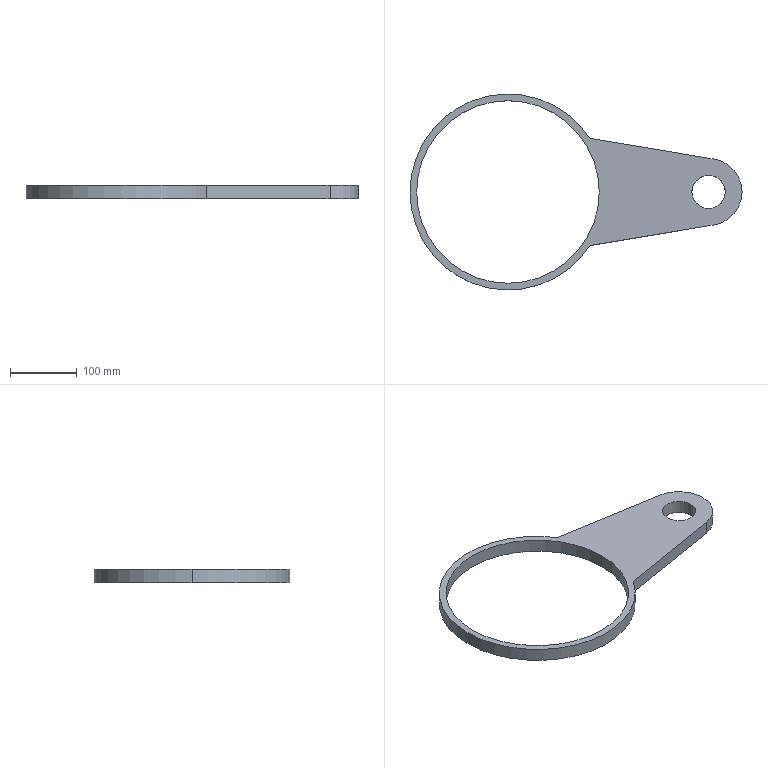Part | SolidWorks | features Extrusion 1 | 1 solid | 11 faces | box 496.5 x 293 x 20 mm | volume 628876 mm3 | cylinder 7 | plane 4 | commonest cylinder face diameters 50 x2 273 x2 293 x2 100 x1
STEP:
#1=CARTESIAN_POINT('',(-136.5,0.,20.));
#2=VERTEX_POINT('',#1);
#3=CARTESIAN_POINT('',(136.5,0.,20.));
#4=VERTEX_POINT('',#3);
#5=CARTESIAN_POINT('',(0.,0.,20.));
#6=DIRECTION('',(0.,0.,1.));
#7=DIRECTION('',(1.,0.,0.));
#8=AXIS2_PLACEMENT_3D('',#5,#6,#7);
#9=CIRCLE('',#8,136.5);
#10=EDGE_CURVE('',#2,#4,#9,.T.);
#11=ORIENTED_EDGE('',*,*,#10,.T.);
#12=CARTESIAN_POINT('',(136.5,0.,0.));
#13=VERTEX_POINT('',#12);
#14=CARTESIAN_POINT('',(136.5,0.,20.));
#15=DIRECTION('',(0.,0.,-1.));
#16=VECTOR('',#15,1000.);
#17=LINE('',#14,#16);
#18=EDGE_CURVE('',#4,#13,#17,.T.);
#19=ORIENTED_EDGE('',*,*,#18,.T.);
#20=CARTESIAN_POINT('',(-136.5,0.,0.));
#21=VERTEX_POINT('',#20);
#22=CARTESIAN_POINT('',(0.,0.,0.));
#23=DIRECTION('',(0.,0.,1.));
#24=DIRECTION('',(1.,0.,0.));
#25=AXIS2_PLACEMENT_3D('',#22,#23,#24);
#26=CIRCLE('',#25,136.5);
#27=EDGE_CURVE('',#21,#13,#26,.T.);
#28=ORIENTED_EDGE('',*,*,#27,.F.);
#29=CARTESIAN_POINT('',(-136.5,0.,20.));
#30=DIRECTION('',(0.,0.,-1.));
#31=VECTOR('',#30,1000.);
#32=LINE('',#29,#31);
#33=EDGE_CURVE('',#2,#21,#32,.T.);
#34=ORIENTED_EDGE('',*,*,#33,.F.);
#35=EDGE_LOOP('',(#11,#19,#28,#34));
#36=FACE_OUTER_BOUND('',#35,.T.);
#37=CARTESIAN_POINT('',(0.,0.,20.));
#38=DIRECTION('',(0.,0.,-1.));
#39=DIRECTION('',(-1.,0.,0.));
#40=AXIS2_PLACEMENT_3D('',#37,#38,#39);
#41=CYLINDRICAL_SURFACE('',#40,136.5);
#42=ADVANCED_FACE('',(#36),#41,.F.);
#43=CARTESIAN_POINT('',(275.,0.,20.));
#44=VERTEX_POINT('',#43);
#45=CARTESIAN_POINT('',(325.,0.,20.));
#46=VERTEX_POINT('',#45);
#47=CARTESIAN_POINT('',(300.,0.,20.));
#48=DIRECTION('',(0.,0.,1.));
#49=DIRECTION('',(1.,0.,0.));
#50=AXIS2_PLACEMENT_3D('',#47,#48,#49);
#51=CIRCLE('',#50,25.);
#52=EDGE_CURVE('',#44,#46,#51,.T.);
#53=ORIENTED_EDGE('',*,*,#52,.T.);
#54=CARTESIAN_POINT('',(325.,0.,0.));
#55=VERTEX_POINT('',#54);
#56=CARTESIAN_POINT('',(325.,0.,20.));
#57=DIRECTION('',(0.,0.,-1.));
#58=VECTOR('',#57,1000.);
#59=LINE('',#56,#58);
#60=EDGE_CURVE('',#46,#55,#59,.T.);
#61=ORIENTED_EDGE('',*,*,#60,.T.);
#62=CARTESIAN_POINT('',(275.,0.,0.));
#63=VERTEX_POINT('',#62);
#64=CARTESIAN_POINT('',(300.,0.,0.));
#65=DIRECTION('',(0.,0.,1.));
#66=DIRECTION('',(1.,0.,0.));
#67=AXIS2_PLACEMENT_3D('',#64,#65,#66);
#68=CIRCLE('',#67,25.);
#69=EDGE_CURVE('',#63,#55,#68,.T.);
#70=ORIENTED_EDGE('',*,*,#69,.F.);
#71=CARTESIAN_POINT('',(275.,0.,20.));
#72=DIRECTION('',(0.,0.,-1.));
#73=VECTOR('',#72,1000.);
#74=LINE('',#71,#73);
#75=EDGE_CURVE('',#44,#63,#74,.T.);
#76=ORIENTED_EDGE('',*,*,#75,.F.);
#77=EDGE_LOOP('',(#53,#61,#70,#76));
#78=FACE_OUTER_BOUND('',#77,.T.);
#79=CARTESIAN_POINT('',(300.,0.,20.));
#80=DIRECTION('',(0.,0.,-1.));
#81=DIRECTION('',(-1.,0.,0.));
#82=AXIS2_PLACEMENT_3D('',#79,#80,#81);
#83=CYLINDRICAL_SURFACE('',#82,25.);
#84=ADVANCED_FACE('',(#78),#83,.F.);
#85=CARTESIAN_POINT('',(-146.5,0.,20.));
#86=VERTEX_POINT('',#85);
#87=CARTESIAN_POINT('',(122.728,-80.,20.));
#88=VERTEX_POINT('',#87);
#89=CARTESIAN_POINT('',(0.,0.,20.));
#90=DIRECTION('',(0.,0.,1.));
#91=DIRECTION('',(1.,0.,0.));
#92=AXIS2_PLACEMENT_3D('',#89,#90,#91);
#93=CIRCLE('',#92,146.5);
#94=EDGE_CURVE('',#86,#88,#93,.T.);
#95=ORIENTED_EDGE('',*,*,#94,.F.);
#96=CARTESIAN_POINT('',(-146.5,0.,0.));
#97=VERTEX_POINT('',#96);
#98=CARTESIAN_POINT('',(-146.5,0.,20.));
#99=DIRECTION('',(0.,0.,-1.));
#100=VECTOR('',#99,1000.);
#101=LINE('',#98,#100);
#102=EDGE_CURVE('',#86,#97,#101,.T.);
#103=ORIENTED_EDGE('',*,*,#102,.T.);
#104=CARTESIAN_POINT('',(122.728,-80.,0.));
#105=VERTEX_POINT('',#104);
#106=CARTESIAN_POINT('',(0.,0.,0.));
#107=DIRECTION('',(0.,0.,1.));
#108=DIRECTION('',(1.,0.,0.));
#109=AXIS2_PLACEMENT_3D('',#106,#107,#108);
#110=CIRCLE('',#109,146.5);
#111=EDGE_CURVE('',#97,#105,#110,.T.);
#112=ORIENTED_EDGE('',*,*,#111,.T.);
#113=CARTESIAN_POINT('',(122.728,-80.,20.));
#114=DIRECTION('',(0.,0.,-1.));
#115=VECTOR('',#114,1000.);
#116=LINE('',#113,#115);
#117=EDGE_CURVE('',#88,#105,#116,.T.);
#118=ORIENTED_EDGE('',*,*,#117,.F.);
#119=EDGE_LOOP('',(#95,#103,#112,#118));
#120=FACE_OUTER_BOUND('',#119,.T.);
#121=CARTESIAN_POINT('',(0.,0.,20.));
#122=DIRECTION('',(0.,0.,-1.));
#123=DIRECTION('',(-1.,0.,0.));
#124=AXIS2_PLACEMENT_3D('',#121,#122,#123);
#125=CYLINDRICAL_SURFACE('',#124,146.5);
#126=ADVANCED_FACE('',(#120),#125,.T.);
#127=ORIENTED_EDGE('',*,*,#52,.F.);
#128=CARTESIAN_POINT('',(300.,0.,20.));
#129=DIRECTION('',(0.,0.,1.));
#130=DIRECTION('',(1.,0.,0.));
#131=AXIS2_PLACEMENT_3D('',#128,#129,#130);
#132=CIRCLE('',#131,25.);
#133=EDGE_CURVE('',#46,#44,#132,.T.);
#134=ORIENTED_EDGE('',*,*,#133,.F.);
#135=EDGE_LOOP('',(#127,#134));
#136=FACE_BOUND('',#135,.T.);
#137=CARTESIAN_POINT('',(122.728,80.,20.));
#138=VERTEX_POINT('',#137);
#139=CARTESIAN_POINT('',(0.,0.,20.));
#140=DIRECTION('',(0.,0.,1.));
#141=DIRECTION('',(1.,0.,0.));
#142=AXIS2_PLACEMENT_3D('',#139,#140,#141);
#143=CIRCLE('',#142,146.5);
#144=EDGE_CURVE('',#138,#86,#143,.T.);
#145=ORIENTED_EDGE('',*,*,#144,.T.);
#146=ORIENTED_EDGE('',*,*,#94,.T.);
#147=CARTESIAN_POINT('',(308.159,-49.33,20.));
#148=VERTEX_POINT('',#147);
#149=CARTESIAN_POINT('',(122.728,-80.,20.));
#150=DIRECTION('',(0.9866,0.1632,0.));
#151=VECTOR('',#150,1000.);
#152=LINE('',#149,#151);
#153=EDGE_CURVE('',#88,#148,#152,.T.);
#154=ORIENTED_EDGE('',*,*,#153,.T.);
#155=CARTESIAN_POINT('',(308.159,49.33,20.));
#156=VERTEX_POINT('',#155);
#157=CARTESIAN_POINT('',(300.,0.,20.));
#158=DIRECTION('',(0.,0.,1.));
#159=DIRECTION('',(1.,0.,0.));
#160=AXIS2_PLACEMENT_3D('',#157,#158,#159);
#161=CIRCLE('',#160,50.);
#162=EDGE_CURVE('',#148,#156,#161,.T.);
#163=ORIENTED_EDGE('',*,*,#162,.T.);
#164=CARTESIAN_POINT('',(122.728,80.,20.));
#165=DIRECTION('',(-0.9866,0.1632,0.));
#166=VECTOR('',#165,1000.);
#167=LINE('',#164,#166);
#168=EDGE_CURVE('',#156,#138,#167,.T.);
#169=ORIENTED_EDGE('',*,*,#168,.T.);
#170=EDGE_LOOP('',(#145,#146,#154,#163,#169));
#171=FACE_OUTER_BOUND('',#170,.T.);
#172=ORIENTED_EDGE('',*,*,#10,.F.);
#173=CARTESIAN_POINT('',(0.,0.,20.));
#174=DIRECTION('',(0.,0.,1.));
#175=DIRECTION('',(1.,0.,0.));
#176=AXIS2_PLACEMENT_3D('',#173,#174,#175);
#177=CIRCLE('',#176,136.5);
#178=EDGE_CURVE('',#4,#2,#177,.T.);
#179=ORIENTED_EDGE('',*,*,#178,.F.);
#180=EDGE_LOOP('',(#172,#179));
#181=FACE_BOUND('',#180,.T.);
#182=CARTESIAN_POINT('',(0.,0.,20.));
#183=DIRECTION('',(0.,0.,1.));
#184=DIRECTION('',(1.,0.,0.));
#185=AXIS2_PLACEMENT_3D('',#182,#183,#184);
#186=PLANE('',#185);
#187=ADVANCED_FACE('',(#136,#171,#181),#186,.T.);
#188=CARTESIAN_POINT('',(122.728,80.,0.));
#189=VERTEX_POINT('',#188);
#190=CARTESIAN_POINT('',(0.,0.,0.));
#191=DIRECTION('',(0.,0.,1.));
#192=DIRECTION('',(1.,0.,0.));
#193=AXIS2_PLACEMENT_3D('',#190,#191,#192);
#194=CIRCLE('',#193,146.5);
#195=EDGE_CURVE('',#189,#97,#194,.T.);
#196=ORIENTED_EDGE('',*,*,#195,.F.);
#197=CARTESIAN_POINT('',(308.159,49.33,0.));
#198=VERTEX_POINT('',#197);
#199=CARTESIAN_POINT('',(122.728,80.,0.));
#200=DIRECTION('',(-0.9866,0.1632,0.));
#201=VECTOR('',#200,1000.);
#202=LINE('',#199,#201);
#203=EDGE_CURVE('',#198,#189,#202,.T.);
#204=ORIENTED_EDGE('',*,*,#203,.F.);
#205=CARTESIAN_POINT('',(308.159,-49.33,0.));
#206=VERTEX_POINT('',#205);
#207=CARTESIAN_POINT('',(300.,0.,0.));
#208=DIRECTION('',(0.,0.,1.));
#209=DIRECTION('',(1.,0.,0.));
#210=AXIS2_PLACEMENT_3D('',#207,#208,#209);
#211=CIRCLE('',#210,50.);
#212=EDGE_CURVE('',#206,#198,#211,.T.);
#213=ORIENTED_EDGE('',*,*,#212,.F.);
#214=CARTESIAN_POINT('',(122.728,-80.,0.));
#215=DIRECTION('',(0.9866,0.1632,0.));
#216=VECTOR('',#215,1000.);
#217=LINE('',#214,#216);
#218=EDGE_CURVE('',#105,#206,#217,.T.);
#219=ORIENTED_EDGE('',*,*,#218,.F.);
#220=ORIENTED_EDGE('',*,*,#111,.F.);
#221=EDGE_LOOP('',(#196,#204,#213,#219,#220));
#222=FACE_OUTER_BOUND('',#221,.T.);
#223=ORIENTED_EDGE('',*,*,#69,.T.);
#224=CARTESIAN_POINT('',(300.,0.,0.));
#225=DIRECTION('',(0.,0.,1.));
#226=DIRECTION('',(1.,0.,0.));
#227=AXIS2_PLACEMENT_3D('',#224,#225,#226);
#228=CIRCLE('',#227,25.);
#229=EDGE_CURVE('',#55,#63,#228,.T.);
#230=ORIENTED_EDGE('',*,*,#229,.T.);
#231=EDGE_LOOP('',(#223,#230));
#232=FACE_BOUND('',#231,.T.);
#233=ORIENTED_EDGE('',*,*,#27,.T.);
#234=CARTESIAN_POINT('',(0.,0.,0.));
#235=DIRECTION('',(0.,0.,1.));
#236=DIRECTION('',(1.,0.,0.));
#237=AXIS2_PLACEMENT_3D('',#234,#235,#236);
#238=CIRCLE('',#237,136.5);
#239=EDGE_CURVE('',#13,#21,#238,.T.);
#240=ORIENTED_EDGE('',*,*,#239,.T.);
#241=EDGE_LOOP('',(#233,#240));
#242=FACE_BOUND('',#241,.T.);
#243=CARTESIAN_POINT('',(0.,0.,0.));
#244=DIRECTION('',(0.,0.,1.));
#245=DIRECTION('',(1.,0.,0.));
#246=AXIS2_PLACEMENT_3D('',#243,#244,#245);
#247=PLANE('',#246);
#248=ADVANCED_FACE('',(#222,#232,#242),#247,.F.);
#249=ORIENTED_EDGE('',*,*,#102,.F.);
#250=ORIENTED_EDGE('',*,*,#144,.F.);
#251=CARTESIAN_POINT('',(122.728,80.,20.));
#252=DIRECTION('',(0.,0.,-1.));
#253=VECTOR('',#252,1000.);
#254=LINE('',#251,#253);
#255=EDGE_CURVE('',#138,#189,#254,.T.);
#256=ORIENTED_EDGE('',*,*,#255,.T.);
#257=ORIENTED_EDGE('',*,*,#195,.T.);
#258=EDGE_LOOP('',(#249,#250,#256,#257));
#259=FACE_OUTER_BOUND('',#258,.T.);
#260=CARTESIAN_POINT('',(0.,0.,20.));
#261=DIRECTION('',(0.,0.,-1.));
#262=DIRECTION('',(-1.,0.,0.));
#263=AXIS2_PLACEMENT_3D('',#260,#261,#262);
#264=CYLINDRICAL_SURFACE('',#263,146.5);
#265=ADVANCED_FACE('',(#259),#264,.T.);
#266=ORIENTED_EDGE('',*,*,#218,.T.);
#267=CARTESIAN_POINT('',(308.159,-49.33,20.));
#268=DIRECTION('',(0.,0.,-1.));
#269=VECTOR('',#268,1000.);
#270=LINE('',#267,#269);
#271=EDGE_CURVE('',#148,#206,#270,.T.);
#272=ORIENTED_EDGE('',*,*,#271,.F.);
#273=ORIENTED_EDGE('',*,*,#153,.F.);
#274=ORIENTED_EDGE('',*,*,#117,.T.);
#275=EDGE_LOOP('',(#266,#272,#273,#274));
#276=FACE_OUTER_BOUND('',#275,.T.);
#277=CARTESIAN_POINT('',(122.728,-80.,20.));
#278=DIRECTION('',(-0.1632,0.9866,0.));
#279=DIRECTION('',(-0.9866,-0.1632,0.));
#280=AXIS2_PLACEMENT_3D('',#277,#278,#279);
#281=PLANE('',#280);
#282=ADVANCED_FACE('',(#276),#281,.F.);
#283=ORIENTED_EDGE('',*,*,#212,.T.);
#284=CARTESIAN_POINT('',(308.159,49.33,20.));
#285=DIRECTION('',(0.,0.,-1.));
#286=VECTOR('',#285,1000.);
#287=LINE('',#284,#286);
#288=EDGE_CURVE('',#156,#198,#287,.T.);
#289=ORIENTED_EDGE('',*,*,#288,.F.);
#290=ORIENTED_EDGE('',*,*,#162,.F.);
#291=ORIENTED_EDGE('',*,*,#271,.T.);
#292=EDGE_LOOP('',(#283,#289,#290,#291));
#293=FACE_OUTER_BOUND('',#292,.T.);
#294=CARTESIAN_POINT('',(300.,0.,20.));
#295=DIRECTION('',(0.,0.,-1.));
#296=DIRECTION('',(-1.,0.,0.));
#297=AXIS2_PLACEMENT_3D('',#294,#295,#296);
#298=CYLINDRICAL_SURFACE('',#297,50.);
#299=ADVANCED_FACE('',(#293),#298,.T.);
#300=ORIENTED_EDGE('',*,*,#203,.T.);
#301=ORIENTED_EDGE('',*,*,#255,.F.);
#302=ORIENTED_EDGE('',*,*,#168,.F.);
#303=ORIENTED_EDGE('',*,*,#288,.T.);
#304=EDGE_LOOP('',(#300,#301,#302,#303));
#305=FACE_OUTER_BOUND('',#304,.T.);
#306=CARTESIAN_POINT('',(122.728,80.,20.));
#307=DIRECTION('',(-0.1632,-0.9866,0.));
#308=DIRECTION('',(0.9866,-0.1632,0.));
#309=AXIS2_PLACEMENT_3D('',#306,#307,#308);
#310=PLANE('',#309);
#311=ADVANCED_FACE('',(#305),#310,.F.);
#312=ORIENTED_EDGE('',*,*,#60,.F.);
#313=ORIENTED_EDGE('',*,*,#133,.T.);
#314=ORIENTED_EDGE('',*,*,#75,.T.);
#315=ORIENTED_EDGE('',*,*,#229,.F.);
#316=EDGE_LOOP('',(#312,#313,#314,#315));
#317=FACE_OUTER_BOUND('',#316,.T.);
#318=CARTESIAN_POINT('',(300.,0.,20.));
#319=DIRECTION('',(0.,0.,-1.));
#320=DIRECTION('',(-1.,0.,0.));
#321=AXIS2_PLACEMENT_3D('',#318,#319,#320);
#322=CYLINDRICAL_SURFACE('',#321,25.);
#323=ADVANCED_FACE('',(#317),#322,.F.);
#324=ORIENTED_EDGE('',*,*,#18,.F.);
#325=ORIENTED_EDGE('',*,*,#178,.T.);
#326=ORIENTED_EDGE('',*,*,#33,.T.);
#327=ORIENTED_EDGE('',*,*,#239,.F.);
#328=EDGE_LOOP('',(#324,#325,#326,#327));
#329=FACE_OUTER_BOUND('',#328,.T.);
#330=CARTESIAN_POINT('',(0.,0.,20.));
#331=DIRECTION('',(0.,0.,-1.));
#332=DIRECTION('',(-1.,0.,0.));
#333=AXIS2_PLACEMENT_3D('',#330,#331,#332);
#334=CYLINDRICAL_SURFACE('',#333,136.5);
#335=ADVANCED_FACE('',(#329),#334,.F.);
#336=CLOSED_SHELL('',(#42,#84,#126,#187,#248,#265,#282,#299,#311,#323,#335));
#337=MANIFOLD_SOLID_BREP('',#336);
#338=CARTESIAN_POINT('',(0.,0.,0.));
#339=DIRECTION('',(0.,0.,1.));
#340=DIRECTION('',(1.,0.,0.));
#341=AXIS2_PLACEMENT_3D('',#338,#339,#340);
#342=(LENGTH_UNIT()NAMED_UNIT(*)SI_UNIT(.MILLI.,.METRE.));
#343=UNCERTAINTY_MEASURE_WITH_UNIT(LENGTH_MEASURE(0.00001),#342,'','');
#344=(NAMED_UNIT(*)PLANE_ANGLE_UNIT()SI_UNIT($,.RADIAN.));
#345=(NAMED_UNIT(*)SI_UNIT($,.STERADIAN.)SOLID_ANGLE_UNIT());
#346=(GEOMETRIC_REPRESENTATION_CONTEXT(3)GLOBAL_UNCERTAINTY_ASSIGNED_CONTEXT((#343))GLOBAL_UNIT_ASSIGNED_CONTEXT((#342,#344,#345))REPRESENTATION_CONTEXT('',''));
#347=ADVANCED_BREP_SHAPE_REPRESENTATION('',(#337,#341),#346);